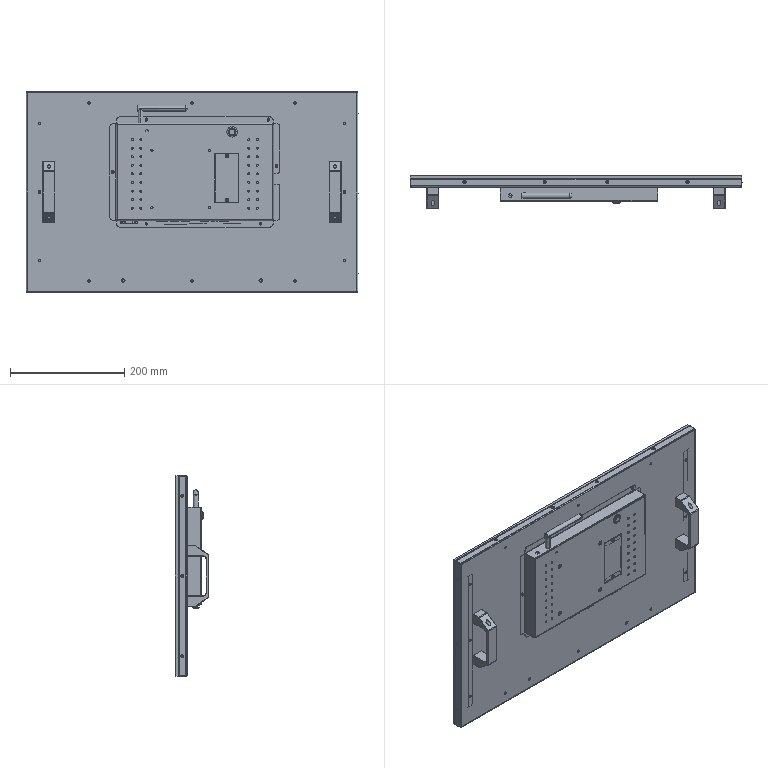Part | SolidWorks | features AEMSimFeature 1 | 20 solids | 1690 faces | box 580.3 x 59 x 351.2 mm | volume 2110380 mm3 | plane 923 | cylinder 639 | spline 116 | cone 10 | torus 2 | commonest cylinder face diameters 3 x94 3.5 x88 5 x79 4 x77 1 x36 6 x24